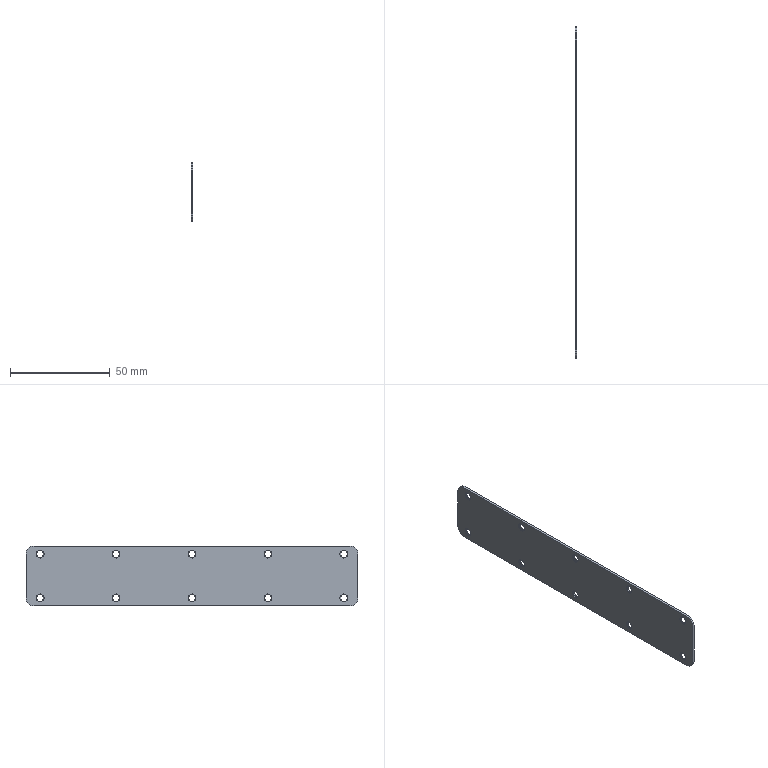Part | STEP file | RJWD-DY-0112_X2_4F20611F56685_1 | 1 solid | 54 faces | box 1 x 166 x 30 mm | volume 4869 mm3 | cone 24 | cylinder 24 | plane 6 | commonest cylinder face diameters 3.4 x20 8 x4